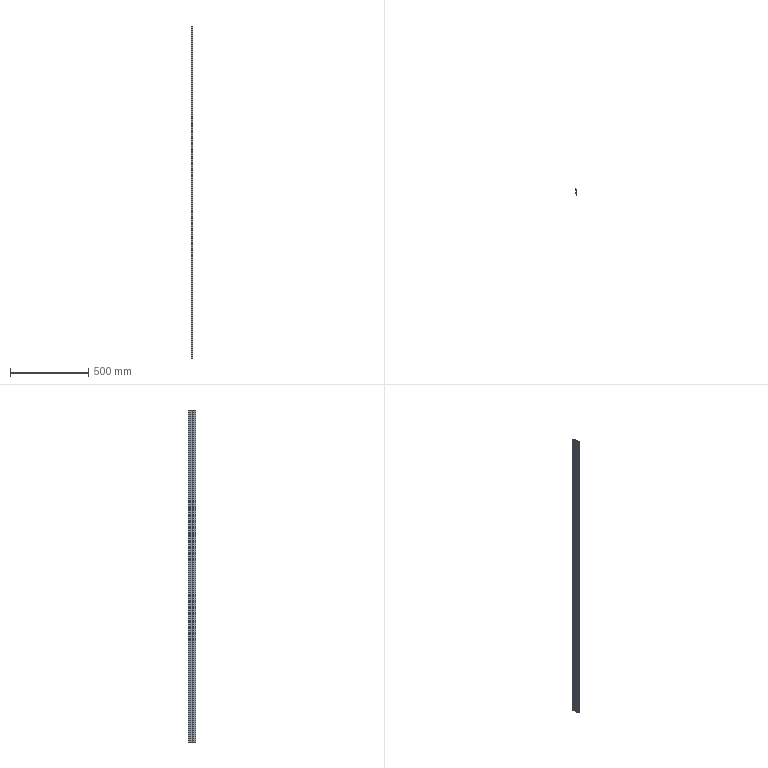Part | SolidWorks | features Extrusion 1 | 1 solid | 33 faces | box 9.4 x 46.998 x 2116 mm | volume 239025 mm3 | plane 22 | cylinder 11 | commonest cylinder face diameters 0.24 x2 0.4 x2 0.8 x2 1.2 x2 6 x2 1 x1
STEP:
#1=CARTESIAN_POINT('',(-2.9,32.45,-1058.));
#2=VERTEX_POINT('',#1);
#3=CARTESIAN_POINT('',(-2.7,32.25,-1058.));
#4=VERTEX_POINT('',#3);
#5=CARTESIAN_POINT('',(-2.7,32.45,-1058.));
#6=DIRECTION('',(0.,0.,1.));
#7=DIRECTION('',(1.,0.,0.));
#8=AXIS2_PLACEMENT_3D('',#5,#6,#7);
#9=CIRCLE('',#8,0.2);
#10=EDGE_CURVE('',#2,#4,#9,.T.);
#11=ORIENTED_EDGE('',*,*,#10,.T.);
#12=CARTESIAN_POINT('',(-2.7,32.25,1058.));
#13=VERTEX_POINT('',#12);
#14=CARTESIAN_POINT('',(-2.7,32.25,1058.));
#15=DIRECTION('',(0.,0.,-1.));
#16=VECTOR('',#15,1000.);
#17=LINE('',#14,#16);
#18=EDGE_CURVE('',#13,#4,#17,.T.);
#19=ORIENTED_EDGE('',*,*,#18,.F.);
#20=CARTESIAN_POINT('',(-2.9,32.45,1058.));
#21=VERTEX_POINT('',#20);
#22=CARTESIAN_POINT('',(-2.7,32.45,1058.));
#23=DIRECTION('',(0.,0.,1.));
#24=DIRECTION('',(1.,0.,0.));
#25=AXIS2_PLACEMENT_3D('',#22,#23,#24);
#26=CIRCLE('',#25,0.2);
#27=EDGE_CURVE('',#21,#13,#26,.T.);
#28=ORIENTED_EDGE('',*,*,#27,.F.);
#29=CARTESIAN_POINT('',(-2.9,32.45,1058.));
#30=DIRECTION('',(0.,0.,-1.));
#31=VECTOR('',#30,1000.);
#32=LINE('',#29,#31);
#33=EDGE_CURVE('',#21,#2,#32,.T.);
#34=ORIENTED_EDGE('',*,*,#33,.T.);
#35=EDGE_LOOP('',(#11,#19,#28,#34));
#36=FACE_OUTER_BOUND('',#35,.T.);
#37=CARTESIAN_POINT('',(-2.7,32.45,1058.));
#38=DIRECTION('',(0.,0.,-1.));
#39=DIRECTION('',(-1.,0.,0.));
#40=AXIS2_PLACEMENT_3D('',#37,#38,#39);
#41=CYLINDRICAL_SURFACE('',#40,0.2);
#42=ADVANCED_FACE('',(#36),#41,.T.);
#43=CARTESIAN_POINT('',(-2.5,32.25,-1058.));
#44=VERTEX_POINT('',#43);
#45=CARTESIAN_POINT('',(-2.7,32.25,-1058.));
#46=DIRECTION('',(1.,0.,0.));
#47=VECTOR('',#46,1000.);
#48=LINE('',#45,#47);
#49=EDGE_CURVE('',#4,#44,#48,.T.);
#50=ORIENTED_EDGE('',*,*,#49,.T.);
#51=CARTESIAN_POINT('',(-2.5,32.25,1058.));
#52=VERTEX_POINT('',#51);
#53=CARTESIAN_POINT('',(-2.5,32.25,1058.));
#54=DIRECTION('',(0.,0.,-1.));
#55=VECTOR('',#54,1000.);
#56=LINE('',#53,#55);
#57=EDGE_CURVE('',#52,#44,#56,.T.);
#58=ORIENTED_EDGE('',*,*,#57,.F.);
#59=CARTESIAN_POINT('',(-2.7,32.25,1058.));
#60=DIRECTION('',(1.,0.,0.));
#61=VECTOR('',#60,1000.);
#62=LINE('',#59,#61);
#63=EDGE_CURVE('',#13,#52,#62,.T.);
#64=ORIENTED_EDGE('',*,*,#63,.F.);
#65=ORIENTED_EDGE('',*,*,#18,.T.);
#66=EDGE_LOOP('',(#50,#58,#64,#65));
#67=FACE_OUTER_BOUND('',#66,.T.);
#68=CARTESIAN_POINT('',(-2.7,32.25,1058.));
#69=DIRECTION('',(0.,1.,0.));
#70=DIRECTION('',(0.,0.,1.));
#71=AXIS2_PLACEMENT_3D('',#68,#69,#70);
#72=PLANE('',#71);
#73=ADVANCED_FACE('',(#67),#72,.F.);
#74=CARTESIAN_POINT('',(-1.9,32.85,-1058.));
#75=VERTEX_POINT('',#74);
#76=CARTESIAN_POINT('',(-2.5,32.85,-1058.));
#77=DIRECTION('',(0.,0.,1.));
#78=DIRECTION('',(1.,0.,0.));
#79=AXIS2_PLACEMENT_3D('',#76,#77,#78);
#80=CIRCLE('',#79,0.6);
#81=EDGE_CURVE('',#44,#75,#80,.T.);
#82=ORIENTED_EDGE('',*,*,#81,.T.);
#83=CARTESIAN_POINT('',(-1.9,32.85,1058.));
#84=VERTEX_POINT('',#83);
#85=CARTESIAN_POINT('',(-1.9,32.85,1058.));
#86=DIRECTION('',(0.,0.,-1.));
#87=VECTOR('',#86,1000.);
#88=LINE('',#85,#87);
#89=EDGE_CURVE('',#84,#75,#88,.T.);
#90=ORIENTED_EDGE('',*,*,#89,.F.);
#91=CARTESIAN_POINT('',(-2.5,32.85,1058.));
#92=DIRECTION('',(0.,0.,1.));
#93=DIRECTION('',(1.,0.,0.));
#94=AXIS2_PLACEMENT_3D('',#91,#92,#93);
#95=CIRCLE('',#94,0.6);
#96=EDGE_CURVE('',#52,#84,#95,.T.);
#97=ORIENTED_EDGE('',*,*,#96,.F.);
#98=ORIENTED_EDGE('',*,*,#57,.T.);
#99=EDGE_LOOP('',(#82,#90,#97,#98));
#100=FACE_OUTER_BOUND('',#99,.T.);
#101=CARTESIAN_POINT('',(-2.5,32.85,1058.));
#102=DIRECTION('',(0.,0.,-1.));
#103=DIRECTION('',(-1.,0.,0.));
#104=AXIS2_PLACEMENT_3D('',#101,#102,#103);
#105=CYLINDRICAL_SURFACE('',#104,0.6);
#106=ADVANCED_FACE('',(#100),#105,.T.);
#107=CARTESIAN_POINT('',(-1.9,36.13,-1058.));
#108=VERTEX_POINT('',#107);
#109=CARTESIAN_POINT('',(-1.9,32.85,-1058.));
#110=DIRECTION('',(0.,1.,0.));
#111=VECTOR('',#110,1000.);
#112=LINE('',#109,#111);
#113=EDGE_CURVE('',#75,#108,#112,.T.);
#114=ORIENTED_EDGE('',*,*,#113,.T.);
#115=CARTESIAN_POINT('',(-1.9,36.13,1058.));
#116=VERTEX_POINT('',#115);
#117=CARTESIAN_POINT('',(-1.9,36.13,1058.));
#118=DIRECTION('',(0.,0.,-1.));
#119=VECTOR('',#118,1000.);
#120=LINE('',#117,#119);
#121=EDGE_CURVE('',#116,#108,#120,.T.);
#122=ORIENTED_EDGE('',*,*,#121,.F.);
#123=CARTESIAN_POINT('',(-1.9,32.85,1058.));
#124=DIRECTION('',(0.,1.,0.));
#125=VECTOR('',#124,1000.);
#126=LINE('',#123,#125);
#127=EDGE_CURVE('',#84,#116,#126,.T.);
#128=ORIENTED_EDGE('',*,*,#127,.F.);
#129=ORIENTED_EDGE('',*,*,#89,.T.);
#130=EDGE_LOOP('',(#114,#122,#128,#129));
#131=FACE_OUTER_BOUND('',#130,.T.);
#132=CARTESIAN_POINT('',(-1.9,32.85,1058.));
#133=DIRECTION('',(-1.,0.,0.));
#134=DIRECTION('',(0.,0.,1.));
#135=AXIS2_PLACEMENT_3D('',#132,#133,#134);
#136=PLANE('',#135);
#137=ADVANCED_FACE('',(#131),#136,.F.);
#138=CARTESIAN_POINT('',(-1.78,36.25,-1058.));
#139=VERTEX_POINT('',#138);
#140=CARTESIAN_POINT('',(-1.78,36.13,-1058.));
#141=DIRECTION('',(0.,0.,-1.));
#142=DIRECTION('',(1.,0.,0.));
#143=AXIS2_PLACEMENT_3D('',#140,#141,#142);
#144=CIRCLE('',#143,0.12);
#145=EDGE_CURVE('',#108,#139,#144,.T.);
#146=ORIENTED_EDGE('',*,*,#145,.T.);
#147=CARTESIAN_POINT('',(-1.78,36.25,1058.));
#148=VERTEX_POINT('',#147);
#149=CARTESIAN_POINT('',(-1.78,36.25,1058.));
#150=DIRECTION('',(0.,0.,-1.));
#151=VECTOR('',#150,1000.);
#152=LINE('',#149,#151);
#153=EDGE_CURVE('',#148,#139,#152,.T.);
#154=ORIENTED_EDGE('',*,*,#153,.F.);
#155=CARTESIAN_POINT('',(-1.78,36.13,1058.));
#156=DIRECTION('',(0.,0.,-1.));
#157=DIRECTION('',(1.,0.,0.));
#158=AXIS2_PLACEMENT_3D('',#155,#156,#157);
#159=CIRCLE('',#158,0.12);
#160=EDGE_CURVE('',#116,#148,#159,.T.);
#161=ORIENTED_EDGE('',*,*,#160,.F.);
#162=ORIENTED_EDGE('',*,*,#121,.T.);
#163=EDGE_LOOP('',(#146,#154,#161,#162));
#164=FACE_OUTER_BOUND('',#163,.T.);
#165=CARTESIAN_POINT('',(-1.78,36.13,1058.));
#166=DIRECTION('',(0.,0.,-1.));
#167=DIRECTION('',(-1.,0.,0.));
#168=AXIS2_PLACEMENT_3D('',#165,#166,#167);
#169=CYLINDRICAL_SURFACE('',#168,0.12);
#170=ADVANCED_FACE('',(#164),#169,.F.);
#171=CARTESIAN_POINT('',(0.,36.25,-1058.));
#172=VERTEX_POINT('',#171);
#173=CARTESIAN_POINT('',(-1.78,36.25,-1058.));
#174=DIRECTION('',(1.,0.,0.));
#175=VECTOR('',#174,1000.);
#176=LINE('',#173,#175);
#177=EDGE_CURVE('',#139,#172,#176,.T.);
#178=ORIENTED_EDGE('',*,*,#177,.T.);
#179=CARTESIAN_POINT('',(0.,36.25,1058.));
#180=VERTEX_POINT('',#179);
#181=CARTESIAN_POINT('',(0.,36.25,1058.));
#182=DIRECTION('',(0.,0.,-1.));
#183=VECTOR('',#182,1000.);
#184=LINE('',#181,#183);
#185=EDGE_CURVE('',#180,#172,#184,.T.);
#186=ORIENTED_EDGE('',*,*,#185,.F.);
#187=CARTESIAN_POINT('',(-1.78,36.25,1058.));
#188=DIRECTION('',(1.,0.,0.));
#189=VECTOR('',#188,1000.);
#190=LINE('',#187,#189);
#191=EDGE_CURVE('',#148,#180,#190,.T.);
#192=ORIENTED_EDGE('',*,*,#191,.F.);
#193=ORIENTED_EDGE('',*,*,#153,.T.);
#194=EDGE_LOOP('',(#178,#186,#192,#193));
#195=FACE_OUTER_BOUND('',#194,.T.);
#196=CARTESIAN_POINT('',(-1.78,36.25,1058.));
#197=DIRECTION('',(0.,1.,0.));
#198=DIRECTION('',(0.,0.,1.));
#199=AXIS2_PLACEMENT_3D('',#196,#197,#198);
#200=PLANE('',#199);
#201=ADVANCED_FACE('',(#195),#200,.F.);
#202=CARTESIAN_POINT('',(0.0007641,20.449,-1058.));
#203=VERTEX_POINT('',#202);
#204=CARTESIAN_POINT('',(0.,36.25,-1058.));
#205=DIRECTION('',(0.00004836,-1.,0.));
#206=VECTOR('',#205,1000.);
#207=LINE('',#204,#206);
#208=EDGE_CURVE('',#172,#203,#207,.T.);
#209=ORIENTED_EDGE('',*,*,#208,.T.);
#210=CARTESIAN_POINT('',(0.0007641,20.449,1058.));
#211=VERTEX_POINT('',#210);
#212=CARTESIAN_POINT('',(0.0007641,20.449,1058.));
#213=DIRECTION('',(0.,0.,-1.));
#214=VECTOR('',#213,1000.);
#215=LINE('',#212,#214);
#216=EDGE_CURVE('',#211,#203,#215,.T.);
#217=ORIENTED_EDGE('',*,*,#216,.F.);
#218=CARTESIAN_POINT('',(0.,36.25,1058.));
#219=DIRECTION('',(0.00004836,-1.,0.));
#220=VECTOR('',#219,1000.);
#221=LINE('',#218,#220);
#222=EDGE_CURVE('',#180,#211,#221,.T.);
#223=ORIENTED_EDGE('',*,*,#222,.F.);
#224=ORIENTED_EDGE('',*,*,#185,.T.);
#225=EDGE_LOOP('',(#209,#217,#223,#224));
#226=FACE_OUTER_BOUND('',#225,.T.);
#227=CARTESIAN_POINT('',(0.,36.25,1058.));
#228=DIRECTION('',(1.,0.00004836,0.));
#229=DIRECTION('',(-0.00004836,1.,0.));
#230=AXIS2_PLACEMENT_3D('',#227,#228,#229);
#231=PLANE('',#230);
#232=ADVANCED_FACE('',(#226),#231,.F.);
#233=CARTESIAN_POINT('',(-2.499,20.449,-1058.));
#234=VERTEX_POINT('',#233);
#235=CARTESIAN_POINT('',(0.0007641,20.449,-1058.));
#236=DIRECTION('',(-1.,0.,0.));
#237=VECTOR('',#236,1000.);
#238=LINE('',#235,#237);
#239=EDGE_CURVE('',#203,#234,#238,.T.);
#240=ORIENTED_EDGE('',*,*,#239,.T.);
#241=CARTESIAN_POINT('',(-2.499,20.449,1058.));
#242=VERTEX_POINT('',#241);
#243=CARTESIAN_POINT('',(-2.499,20.449,1058.));
#244=DIRECTION('',(0.,0.,-1.));
#245=VECTOR('',#244,1000.);
#246=LINE('',#243,#245);
#247=EDGE_CURVE('',#242,#234,#246,.T.);
#248=ORIENTED_EDGE('',*,*,#247,.F.);
#249=CARTESIAN_POINT('',(0.0007641,20.449,1058.));
#250=DIRECTION('',(-1.,0.,0.));
#251=VECTOR('',#250,1000.);
#252=LINE('',#249,#251);
#253=EDGE_CURVE('',#211,#242,#252,.T.);
#254=ORIENTED_EDGE('',*,*,#253,.F.);
#255=ORIENTED_EDGE('',*,*,#216,.T.);
#256=EDGE_LOOP('',(#240,#248,#254,#255));
#257=FACE_OUTER_BOUND('',#256,.T.);
#258=CARTESIAN_POINT('',(0.0007641,20.449,1058.));
#259=DIRECTION('',(0.,-1.,0.));
#260=DIRECTION('',(0.,0.,-1.));
#261=AXIS2_PLACEMENT_3D('',#258,#259,#260);
#262=PLANE('',#261);
#263=ADVANCED_FACE('',(#257),#262,.F.);
#264=CARTESIAN_POINT('',(-2.899,20.049,-1058.));
#265=VERTEX_POINT('',#264);
#266=CARTESIAN_POINT('',(-2.499,20.049,-1058.));
#267=DIRECTION('',(0.,0.,1.));
#268=DIRECTION('',(1.,0.,0.));
#269=AXIS2_PLACEMENT_3D('',#266,#267,#268);
#270=CIRCLE('',#269,0.4);
#271=EDGE_CURVE('',#234,#265,#270,.T.);
#272=ORIENTED_EDGE('',*,*,#271,.T.);
#273=CARTESIAN_POINT('',(-2.899,20.049,1058.));
#274=VERTEX_POINT('',#273);
#275=CARTESIAN_POINT('',(-2.899,20.049,1058.));
#276=DIRECTION('',(0.,0.,-1.));
#277=VECTOR('',#276,1000.);
#278=LINE('',#275,#277);
#279=EDGE_CURVE('',#274,#265,#278,.T.);
#280=ORIENTED_EDGE('',*,*,#279,.F.);
#281=CARTESIAN_POINT('',(-2.499,20.049,1058.));
#282=DIRECTION('',(0.,0.,1.));
#283=DIRECTION('',(1.,0.,0.));
#284=AXIS2_PLACEMENT_3D('',#281,#282,#283);
#285=CIRCLE('',#284,0.4);
#286=EDGE_CURVE('',#242,#274,#285,.T.);
#287=ORIENTED_EDGE('',*,*,#286,.F.);
#288=ORIENTED_EDGE('',*,*,#247,.T.);
#289=EDGE_LOOP('',(#272,#280,#287,#288));
#290=FACE_OUTER_BOUND('',#289,.T.);
#291=CARTESIAN_POINT('',(-2.499,20.049,1058.));
#292=DIRECTION('',(0.,0.,-1.));
#293=DIRECTION('',(-1.,0.,0.));
#294=AXIS2_PLACEMENT_3D('',#291,#292,#293);
#295=CYLINDRICAL_SURFACE('',#294,0.4);
#296=ADVANCED_FACE('',(#290),#295,.T.);
#297=CARTESIAN_POINT('',(-2.899,15.65,-1058.));
#298=VERTEX_POINT('',#297);
#299=CARTESIAN_POINT('',(-2.899,20.049,-1058.));
#300=DIRECTION('',(0.,-1.,0.));
#301=VECTOR('',#300,1000.);
#302=LINE('',#299,#301);
#303=EDGE_CURVE('',#265,#298,#302,.T.);
#304=ORIENTED_EDGE('',*,*,#303,.T.);
#305=CARTESIAN_POINT('',(-2.899,15.65,1058.));
#306=VERTEX_POINT('',#305);
#307=CARTESIAN_POINT('',(-2.899,15.65,1058.));
#308=DIRECTION('',(0.,0.,-1.));
#309=VECTOR('',#308,1000.);
#310=LINE('',#307,#309);
#311=EDGE_CURVE('',#306,#298,#310,.T.);
#312=ORIENTED_EDGE('',*,*,#311,.F.);
#313=CARTESIAN_POINT('',(-2.899,20.049,1058.));
#314=DIRECTION('',(0.,-1.,0.));
#315=VECTOR('',#314,1000.);
#316=LINE('',#313,#315);
#317=EDGE_CURVE('',#274,#306,#316,.T.);
#318=ORIENTED_EDGE('',*,*,#317,.F.);
#319=ORIENTED_EDGE('',*,*,#279,.T.);
#320=EDGE_LOOP('',(#304,#312,#318,#319));
#321=FACE_OUTER_BOUND('',#320,.T.);
#322=CARTESIAN_POINT('',(-2.899,20.049,1058.));
#323=DIRECTION('',(1.,0.,0.));
#324=DIRECTION('',(0.,0.,-1.));
#325=AXIS2_PLACEMENT_3D('',#322,#323,#324);
#326=PLANE('',#325);
#327=ADVANCED_FACE('',(#321),#326,.F.);
#328=CARTESIAN_POINT('',(-2.699,15.45,-1058.));
#329=VERTEX_POINT('',#328);
#330=CARTESIAN_POINT('',(-2.699,15.65,-1058.));
#331=DIRECTION('',(0.,0.,1.));
#332=DIRECTION('',(1.,0.,0.));
#333=AXIS2_PLACEMENT_3D('',#330,#331,#332);
#334=CIRCLE('',#333,0.2);
#335=EDGE_CURVE('',#298,#329,#334,.T.);
#336=ORIENTED_EDGE('',*,*,#335,.T.);
#337=CARTESIAN_POINT('',(-2.699,15.45,1058.));
#338=VERTEX_POINT('',#337);
#339=CARTESIAN_POINT('',(-2.699,15.45,1058.));
#340=DIRECTION('',(0.,0.,-1.));
#341=VECTOR('',#340,1000.);
#342=LINE('',#339,#341);
#343=EDGE_CURVE('',#338,#329,#342,.T.);
#344=ORIENTED_EDGE('',*,*,#343,.F.);
#345=CARTESIAN_POINT('',(-2.699,15.65,1058.));
#346=DIRECTION('',(0.,0.,1.));
#347=DIRECTION('',(1.,0.,0.));
#348=AXIS2_PLACEMENT_3D('',#345,#346,#347);
#349=CIRCLE('',#348,0.2);
#350=EDGE_CURVE('',#306,#338,#349,.T.);
#351=ORIENTED_EDGE('',*,*,#350,.F.);
#352=ORIENTED_EDGE('',*,*,#311,.T.);
#353=EDGE_LOOP('',(#336,#344,#351,#352));
#354=FACE_OUTER_BOUND('',#353,.T.);
#355=CARTESIAN_POINT('',(-2.699,15.65,1058.));
#356=DIRECTION('',(0.,0.,-1.));
#357=DIRECTION('',(-1.,0.,0.));
#358=AXIS2_PLACEMENT_3D('',#355,#356,#357);
#359=CYLINDRICAL_SURFACE('',#358,0.2);
#360=ADVANCED_FACE('',(#354),#359,.T.);
#361=CARTESIAN_POINT('',(-2.499,15.45,-1058.));
#362=VERTEX_POINT('',#361);
#363=CARTESIAN_POINT('',(-2.699,15.45,-1058.));
#364=DIRECTION('',(1.,0.,0.));
#365=VECTOR('',#364,1000.);
#366=LINE('',#363,#365);
#367=EDGE_CURVE('',#329,#362,#366,.T.);
#368=ORIENTED_EDGE('',*,*,#367,.T.);
#369=CARTESIAN_POINT('',(-2.499,15.45,1058.));
#370=VERTEX_POINT('',#369);
#371=CARTESIAN_POINT('',(-2.499,15.45,1058.));
#372=DIRECTION('',(0.,0.,-1.));
#373=VECTOR('',#372,1000.);
#374=LINE('',#371,#373);
#375=EDGE_CURVE('',#370,#362,#374,.T.);
#376=ORIENTED_EDGE('',*,*,#375,.F.);
#377=CARTESIAN_POINT('',(-2.699,15.45,1058.));
#378=DIRECTION('',(1.,0.,0.));
#379=VECTOR('',#378,1000.);
#380=LINE('',#377,#379);
#381=EDGE_CURVE('',#338,#370,#380,.T.);
#382=ORIENTED_EDGE('',*,*,#381,.F.);
#383=ORIENTED_EDGE('',*,*,#343,.T.);
#384=EDGE_LOOP('',(#368,#376,#382,#383));
#385=FACE_OUTER_BOUND('',#384,.T.);
#386=CARTESIAN_POINT('',(-2.699,15.45,1058.));
#387=DIRECTION('',(0.,1.,0.));
#388=DIRECTION('',(0.,0.,1.));
#389=AXIS2_PLACEMENT_3D('',#386,#387,#388);
#390=PLANE('',#389);
#391=ADVANCED_FACE('',(#385),#390,.F.);
#392=CARTESIAN_POINT('',(-1.899,16.05,-1058.));
#393=VERTEX_POINT('',#392);
#394=CARTESIAN_POINT('',(-2.499,16.05,-1058.));
#395=DIRECTION('',(0.,0.,1.));
#396=DIRECTION('',(1.,0.,0.));
#397=AXIS2_PLACEMENT_3D('',#394,#395,#396);
#398=CIRCLE('',#397,0.6);
#399=EDGE_CURVE('',#362,#393,#398,.T.);
#400=ORIENTED_EDGE('',*,*,#399,.T.);
#401=CARTESIAN_POINT('',(-1.899,16.05,1058.));
#402=VERTEX_POINT('',#401);
#403=CARTESIAN_POINT('',(-1.899,16.05,1058.));
#404=DIRECTION('',(0.,0.,-1.));
#405=VECTOR('',#404,1000.);
#406=LINE('',#403,#405);
#407=EDGE_CURVE('',#402,#393,#406,.T.);
#408=ORIENTED_EDGE('',*,*,#407,.F.);
#409=CARTESIAN_POINT('',(-2.499,16.05,1058.));
#410=DIRECTION('',(0.,0.,1.));
#411=DIRECTION('',(1.,0.,0.));
#412=AXIS2_PLACEMENT_3D('',#409,#410,#411);
#413=CIRCLE('',#412,0.6);
#414=EDGE_CURVE('',#370,#402,#413,.T.);
#415=ORIENTED_EDGE('',*,*,#414,.F.);
#416=ORIENTED_EDGE('',*,*,#375,.T.);
#417=EDGE_LOOP('',(#400,#408,#415,#416));
#418=FACE_OUTER_BOUND('',#417,.T.);
#419=CARTESIAN_POINT('',(-2.499,16.05,1058.));
#420=DIRECTION('',(0.,0.,-1.));
#421=DIRECTION('',(-1.,0.,0.));
#422=AXIS2_PLACEMENT_3D('',#419,#420,#421);
#423=CYLINDRICAL_SURFACE('',#422,0.6);
#424=ADVANCED_FACE('',(#418),#423,.T.);
#425=CARTESIAN_POINT('',(-1.899,19.329,-1058.));
#426=VERTEX_POINT('',#425);
#427=CARTESIAN_POINT('',(-1.899,16.05,-1058.));
#428=DIRECTION('',(0.,1.,0.));
#429=VECTOR('',#428,1000.);
#430=LINE('',#427,#429);
#431=EDGE_CURVE('',#393,#426,#430,.T.);
#432=ORIENTED_EDGE('',*,*,#431,.T.);
#433=CARTESIAN_POINT('',(-1.899,19.329,1058.));
#434=VERTEX_POINT('',#433);
#435=CARTESIAN_POINT('',(-1.899,19.329,1058.));
#436=DIRECTION('',(0.,0.,-1.));
#437=VECTOR('',#436,1000.);
#438=LINE('',#435,#437);
#439=EDGE_CURVE('',#434,#426,#438,.T.);
#440=ORIENTED_EDGE('',*,*,#439,.F.);
#441=CARTESIAN_POINT('',(-1.899,16.05,1058.));
#442=DIRECTION('',(0.,1.,0.));
#443=VECTOR('',#442,1000.);
#444=LINE('',#441,#443);
#445=EDGE_CURVE('',#402,#434,#444,.T.);
#446=ORIENTED_EDGE('',*,*,#445,.F.);
#447=ORIENTED_EDGE('',*,*,#407,.T.);
#448=EDGE_LOOP('',(#432,#440,#446,#447));
#449=FACE_OUTER_BOUND('',#448,.T.);
#450=CARTESIAN_POINT('',(-1.899,16.05,1058.));
#451=DIRECTION('',(-1.,0.,0.));
#452=DIRECTION('',(0.,0.,1.));
#453=AXIS2_PLACEMENT_3D('',#450,#451,#452);
#454=PLANE('',#453);
#455=ADVANCED_FACE('',(#449),#454,.F.);
#456=CARTESIAN_POINT('',(-1.779,19.449,-1058.));
#457=VERTEX_POINT('',#456);
#458=CARTESIAN_POINT('',(-1.779,19.329,-1058.));
#459=DIRECTION('',(0.,0.,-1.));
#460=DIRECTION('',(1.,0.,0.));
#461=AXIS2_PLACEMENT_3D('',#458,#459,#460);
#462=CIRCLE('',#461,0.12);
#463=EDGE_CURVE('',#426,#457,#462,.T.);
#464=ORIENTED_EDGE('',*,*,#463,.T.);
#465=CARTESIAN_POINT('',(-1.779,19.449,1058.));
#466=VERTEX_POINT('',#465);
#467=CARTESIAN_POINT('',(-1.779,19.449,1058.));
#468=DIRECTION('',(0.,0.,-1.));
#469=VECTOR('',#468,1000.);
#470=LINE('',#467,#469);
#471=EDGE_CURVE('',#466,#457,#470,.T.);
#472=ORIENTED_EDGE('',*,*,#471,.F.);
#473=CARTESIAN_POINT('',(-1.779,19.329,1058.));
#474=DIRECTION('',(0.,0.,-1.));
#475=DIRECTION('',(1.,0.,0.));
#476=AXIS2_PLACEMENT_3D('',#473,#474,#475);
#477=CIRCLE('',#476,0.12);
#478=EDGE_CURVE('',#434,#466,#477,.T.);
#479=ORIENTED_EDGE('',*,*,#478,.F.);
#480=ORIENTED_EDGE('',*,*,#439,.T.);
#481=EDGE_LOOP('',(#464,#472,#479,#480));
#482=FACE_OUTER_BOUND('',#481,.T.);
#483=CARTESIAN_POINT('',(-1.779,19.329,1058.));
#484=DIRECTION('',(0.,0.,-1.));
#485=DIRECTION('',(-1.,0.,0.));
#486=AXIS2_PLACEMENT_3D('',#483,#484,#485);
#487=CYLINDRICAL_SURFACE('',#486,0.12);
#488=ADVANCED_FACE('',(#482),#487,.F.);
#489=CARTESIAN_POINT('',(0.0007641,19.449,-1058.));
#490=VERTEX_POINT('',#489);
#491=CARTESIAN_POINT('',(-1.779,19.449,-1058.));
#492=DIRECTION('',(1.,0.,0.));
#493=VECTOR('',#492,1000.);
#494=LINE('',#491,#493);
#495=EDGE_CURVE('',#457,#490,#494,.T.);
#496=ORIENTED_EDGE('',*,*,#495,.T.);
#497=CARTESIAN_POINT('',(0.0007641,19.449,1058.));
#498=VERTEX_POINT('',#497);
#499=CARTESIAN_POINT('',(0.0007641,19.449,1058.));
#500=DIRECTION('',(0.,0.,-1.));
#501=VECTOR('',#500,1000.);
#502=LINE('',#499,#501);
#503=EDGE_CURVE('',#498,#490,#502,.T.);
#504=ORIENTED_EDGE('',*,*,#503,.F.);
#505=CARTESIAN_POINT('',(-1.779,19.449,1058.));
#506=DIRECTION('',(1.,0.,0.));
#507=VECTOR('',#506,1000.);
#508=LINE('',#505,#507);
#509=EDGE_CURVE('',#466,#498,#508,.T.);
#510=ORIENTED_EDGE('',*,*,#509,.F.);
#511=ORIENTED_EDGE('',*,*,#471,.T.);
#512=EDGE_LOOP('',(#496,#504,#510,#511));
#513=FACE_OUTER_BOUND('',#512,.T.);
#514=CARTESIAN_POINT('',(-1.779,19.449,1058.));
#515=DIRECTION('',(0.,1.,0.));
#516=DIRECTION('',(0.,0.,1.));
#517=AXIS2_PLACEMENT_3D('',#514,#515,#516);
#518=PLANE('',#517);
#519=ADVANCED_FACE('',(#513),#518,.F.);
#520=CARTESIAN_POINT('',(0.,0.,-1058.));
#521=VERTEX_POINT('',#520);
#522=CARTESIAN_POINT('',(0.0007641,19.449,-1058.));
#523=DIRECTION('',(-0.00003929,-1.,0.));
#524=VECTOR('',#523,1000.);
#525=LINE('',#522,#524);
#526=EDGE_CURVE('',#490,#521,#525,.T.);
#527=ORIENTED_EDGE('',*,*,#526,.T.);
#528=CARTESIAN_POINT('',(0.,0.,1058.));
#529=VERTEX_POINT('',#528);
#530=CARTESIAN_POINT('',(0.,0.,1058.));
#531=DIRECTION('',(0.,0.,-1.));
#532=VECTOR('',#531,1000.);
#533=LINE('',#530,#532);
#534=EDGE_CURVE('',#529,#521,#533,.T.);
#535=ORIENTED_EDGE('',*,*,#534,.F.);
#536=CARTESIAN_POINT('',(0.0007641,19.449,1058.));
#537=DIRECTION('',(-0.00003929,-1.,0.));
#538=VECTOR('',#537,1000.);
#539=LINE('',#536,#538);
#540=EDGE_CURVE('',#498,#529,#539,.T.);
#541=ORIENTED_EDGE('',*,*,#540,.F.);
#542=ORIENTED_EDGE('',*,*,#503,.T.);
#543=EDGE_LOOP('',(#527,#535,#541,#542));
#544=FACE_OUTER_BOUND('',#543,.T.);
#545=CARTESIAN_POINT('',(0.0007641,19.449,1058.));
#546=DIRECTION('',(1.,-0.00003929,0.));
#547=DIRECTION('',(0.00003929,1.,0.));
#548=AXIS2_PLACEMENT_3D('',#545,#546,#547);
#549=PLANE('',#548);
#550=ADVANCED_FACE('',(#544),#549,.F.);
#551=CARTESIAN_POINT('',(1.5,0.,-1058.));
#552=VERTEX_POINT('',#551);
#553=CARTESIAN_POINT('',(0.,0.,-1058.));
#554=DIRECTION('',(1.,0.,0.));
#555=VECTOR('',#554,1000.);
#556=LINE('',#553,#555);
#557=EDGE_CURVE('',#521,#552,#556,.T.);
#558=ORIENTED_EDGE('',*,*,#557,.T.);
#559=CARTESIAN_POINT('',(1.5,0.,1058.));
#560=VERTEX_POINT('',#559);
#561=CARTESIAN_POINT('',(1.5,0.,1058.));
#562=DIRECTION('',(0.,0.,-1.));
#563=VECTOR('',#562,1000.);
#564=LINE('',#561,#563);
#565=EDGE_CURVE('',#560,#552,#564,.T.);
#566=ORIENTED_EDGE('',*,*,#565,.F.);
#567=CARTESIAN_POINT('',(0.,0.,1058.));
#568=DIRECTION('',(1.,0.,0.));
#569=VECTOR('',#568,1000.);
#570=LINE('',#567,#569);
#571=EDGE_CURVE('',#529,#560,#570,.T.);
#572=ORIENTED_EDGE('',*,*,#571,.F.);
#573=ORIENTED_EDGE('',*,*,#534,.T.);
#574=EDGE_LOOP('',(#558,#566,#572,#573));
#575=FACE_OUTER_BOUND('',#574,.T.);
#576=CARTESIAN_POINT('',(0.,0.,1058.));
#577=DIRECTION('',(0.,1.,0.));
#578=DIRECTION('',(0.,0.,1.));
#579=AXIS2_PLACEMENT_3D('',#576,#577,#578);
#580=PLANE('',#579);
#581=ADVANCED_FACE('',(#575),#580,.F.);
#582=CARTESIAN_POINT('',(2.,0.5,-1058.));
#583=VERTEX_POINT('',#582);
#584=CARTESIAN_POINT('',(1.5,0.5,-1058.));
#585=DIRECTION('',(0.,0.,1.));
#586=DIRECTION('',(1.,0.,0.));
#587=AXIS2_PLACEMENT_3D('',#584,#585,#586);
#588=CIRCLE('',#587,0.5);
#589=EDGE_CURVE('',#552,#583,#588,.T.);
#590=ORIENTED_EDGE('',*,*,#589,.T.);
#591=CARTESIAN_POINT('',(2.,0.5,1058.));
#592=VERTEX_POINT('',#591);
#593=CARTESIAN_POINT('',(2.,0.5,1058.));
#594=DIRECTION('',(0.,0.,-1.));
#595=VECTOR('',#594,1000.);
#596=LINE('',#593,#595);
#597=EDGE_CURVE('',#592,#583,#596,.T.);
#598=ORIENTED_EDGE('',*,*,#597,.F.);
#599=CARTESIAN_POINT('',(1.5,0.5,1058.));
#600=DIRECTION('',(0.,0.,1.));
#601=DIRECTION('',(1.,0.,0.));
#602=AXIS2_PLACEMENT_3D('',#599,#600,#601);
#603=CIRCLE('',#602,0.5);
#604=EDGE_CURVE('',#560,#592,#603,.T.);
#605=ORIENTED_EDGE('',*,*,#604,.F.);
#606=ORIENTED_EDGE('',*,*,#565,.T.);
#607=EDGE_LOOP('',(#590,#598,#605,#606));
#608=FACE_OUTER_BOUND('',#607,.T.);
#609=CARTESIAN_POINT('',(1.5,0.5,1058.));
#610=DIRECTION('',(0.,0.,-1.));
#611=DIRECTION('',(-1.,0.,0.));
#612=AXIS2_PLACEMENT_3D('',#609,#610,#611);
#613=CYLINDRICAL_SURFACE('',#612,0.5);
#614=ADVANCED_FACE('',(#608),#613,.T.);
#615=CARTESIAN_POINT('',(2.,38.058,-1058.));
#616=VERTEX_POINT('',#615);
#617=CARTESIAN_POINT('',(2.,0.5,-1058.));
#618=DIRECTION('',(0.,1.,0.));
#619=VECTOR('',#618,1000.);
#620=LINE('',#617,#619);
#621=EDGE_CURVE('',#583,#616,#620,.T.);
#622=ORIENTED_EDGE('',*,*,#621,.T.);
#623=CARTESIAN_POINT('',(2.,38.058,1058.));
#624=VERTEX_POINT('',#623);
#625=CARTESIAN_POINT('',(2.,38.058,1058.));
#626=DIRECTION('',(0.,0.,-1.));
#627=VECTOR('',#626,1000.);
#628=LINE('',#625,#627);
#629=EDGE_CURVE('',#624,#616,#628,.T.);
#630=ORIENTED_EDGE('',*,*,#629,.F.);
#631=CARTESIAN_POINT('',(2.,0.5,1058.));
#632=DIRECTION('',(0.,1.,0.));
#633=VECTOR('',#632,1000.);
#634=LINE('',#631,#633);
#635=EDGE_CURVE('',#592,#624,#634,.T.);
#636=ORIENTED_EDGE('',*,*,#635,.F.);
#637=ORIENTED_EDGE('',*,*,#597,.T.);
#638=EDGE_LOOP('',(#622,#630,#636,#637));
#639=FACE_OUTER_BOUND('',#638,.T.);
#640=CARTESIAN_POINT('',(2.,0.5,1058.));
#641=DIRECTION('',(-1.,0.,0.));
#642=DIRECTION('',(0.,0.,1.));
#643=AXIS2_PLACEMENT_3D('',#640,#641,#642);
#644=PLANE('',#643);
#645=ADVANCED_FACE('',(#639),#644,.F.);
#646=CARTESIAN_POINT('',(1.393,39.868,-1058.));
#647=VERTEX_POINT('',#646);
#648=CARTESIAN_POINT('',(-1.,38.058,-1058.));
#649=DIRECTION('',(0.,0.,1.));
#650=DIRECTION('',(1.,0.,0.));
#651=AXIS2_PLACEMENT_3D('',#648,#649,#650);
#652=CIRCLE('',#651,3.);
#653=EDGE_CURVE('',#616,#647,#652,.T.);
#654=ORIENTED_EDGE('',*,*,#653,.T.);
#655=CARTESIAN_POINT('',(1.393,39.868,1058.));
#656=VERTEX_POINT('',#655);
#657=CARTESIAN_POINT('',(1.393,39.868,1058.));
#658=DIRECTION('',(0.,0.,-1.));
#659=VECTOR('',#658,1000.);
#660=LINE('',#657,#659);
#661=EDGE_CURVE('',#656,#647,#660,.T.);
#662=ORIENTED_EDGE('',*,*,#661,.F.);
#663=CARTESIAN_POINT('',(-1.,38.058,1058.));
#664=DIRECTION('',(0.,0.,1.));
#665=DIRECTION('',(1.,0.,0.));
#666=AXIS2_PLACEMENT_3D('',#663,#664,#665);
#667=CIRCLE('',#666,3.);
#668=EDGE_CURVE('',#624,#656,#667,.T.);
#669=ORIENTED_EDGE('',*,*,#668,.F.);
#670=ORIENTED_EDGE('',*,*,#629,.T.);
#671=EDGE_LOOP('',(#654,#662,#669,#670));
#672=FACE_OUTER_BOUND('',#671,.T.);
#673=CARTESIAN_POINT('',(-1.,38.058,1058.));
#674=DIRECTION('',(0.,0.,-1.));
#675=DIRECTION('',(-1.,0.,0.));
#676=AXIS2_PLACEMENT_3D('',#673,#674,#675);
#677=CYLINDRICAL_SURFACE('',#676,3.);
#678=ADVANCED_FACE('',(#672),#677,.T.);
#679=CARTESIAN_POINT('',(-4.,46.998,-1058.));
#680=VERTEX_POINT('',#679);
#681=CARTESIAN_POINT('',(1.393,39.868,-1058.));
#682=DIRECTION('',(-0.6032,0.7976,0.));
#683=VECTOR('',#682,1000.);
#684=LINE('',#681,#683);
#685=EDGE_CURVE('',#647,#680,#684,.T.);
#686=ORIENTED_EDGE('',*,*,#685,.T.);
#687=CARTESIAN_POINT('',(-4.,46.998,1058.));
#688=VERTEX_POINT('',#687);
#689=CARTESIAN_POINT('',(-4.,46.998,1058.));
#690=DIRECTION('',(0.,0.,-1.));
#691=VECTOR('',#690,1000.);
#692=LINE('',#689,#691);
#693=EDGE_CURVE('',#688,#680,#692,.T.);
#694=ORIENTED_EDGE('',*,*,#693,.F.);
#695=CARTESIAN_POINT('',(1.393,39.868,1058.));
#696=DIRECTION('',(-0.6032,0.7976,0.));
#697=VECTOR('',#696,1000.);
#698=LINE('',#695,#697);
#699=EDGE_CURVE('',#656,#688,#698,.T.);
#700=ORIENTED_EDGE('',*,*,#699,.F.);
#701=ORIENTED_EDGE('',*,*,#661,.T.);
#702=EDGE_LOOP('',(#686,#694,#700,#701));
#703=FACE_OUTER_BOUND('',#702,.T.);
#704=CARTESIAN_POINT('',(1.393,39.868,1058.));
#705=DIRECTION('',(-0.7976,-0.6032,0.));
#706=DIRECTION('',(0.6032,-0.7976,0.));
#707=AXIS2_PLACEMENT_3D('',#704,#705,#706);
#708=PLANE('',#707);
#709=ADVANCED_FACE('',(#703),#708,.F.);
#710=CARTESIAN_POINT('',(-7.4,46.998,-1058.));
#711=VERTEX_POINT('',#710);
#712=CARTESIAN_POINT('',(-4.,46.998,-1058.));
#713=DIRECTION('',(-1.,0.,0.));
#714=VECTOR('',#713,1000.);
#715=LINE('',#712,#714);
#716=EDGE_CURVE('',#680,#711,#715,.T.);
#717=ORIENTED_EDGE('',*,*,#716,.T.);
#718=CARTESIAN_POINT('',(-7.4,46.998,1058.));
#719=VERTEX_POINT('',#718);
#720=CARTESIAN_POINT('',(-7.4,46.998,1058.));
#721=DIRECTION('',(0.,0.,-1.));
#722=VECTOR('',#721,1000.);
#723=LINE('',#720,#722);
#724=EDGE_CURVE('',#719,#711,#723,.T.);
#725=ORIENTED_EDGE('',*,*,#724,.F.);
#726=CARTESIAN_POINT('',(-4.,46.998,1058.));
#727=DIRECTION('',(-1.,0.,0.));
#728=VECTOR('',#727,1000.);
#729=LINE('',#726,#728);
#730=EDGE_CURVE('',#688,#719,#729,.T.);
#731=ORIENTED_EDGE('',*,*,#730,.F.);
#732=ORIENTED_EDGE('',*,*,#693,.T.);
#733=EDGE_LOOP('',(#717,#725,#731,#732));
#734=FACE_OUTER_BOUND('',#733,.T.);
#735=CARTESIAN_POINT('',(-4.,46.998,1058.));
#736=DIRECTION('',(0.,-1.,0.));
#737=DIRECTION('',(0.,0.,-1.));
#738=AXIS2_PLACEMENT_3D('',#735,#736,#737);
#739=PLANE('',#738);
#740=ADVANCED_FACE('',(#734),#739,.F.);
#741=CARTESIAN_POINT('',(-7.4,45.998,-1058.));
#742=VERTEX_POINT('',#741);
#743=CARTESIAN_POINT('',(-7.4,46.998,-1058.));
#744=DIRECTION('',(0.,-1.,0.));
#745=VECTOR('',#744,1000.);
#746=LINE('',#743,#745);
#747=EDGE_CURVE('',#711,#742,#746,.T.);
#748=ORIENTED_EDGE('',*,*,#747,.T.);
#749=CARTESIAN_POINT('',(-7.4,45.998,1058.));
#750=VERTEX_POINT('',#749);
#751=CARTESIAN_POINT('',(-7.4,45.998,1058.));
#752=DIRECTION('',(0.,0.,-1.));
#753=VECTOR('',#752,1000.);
#754=LINE('',#751,#753);
#755=EDGE_CURVE('',#750,#742,#754,.T.);
#756=ORIENTED_EDGE('',*,*,#755,.F.);
#757=CARTESIAN_POINT('',(-7.4,46.998,1058.));
#758=DIRECTION('',(0.,-1.,0.));
#759=VECTOR('',#758,1000.);
#760=LINE('',#757,#759);
#761=EDGE_CURVE('',#719,#750,#760,.T.);
#762=ORIENTED_EDGE('',*,*,#761,.F.);
#763=ORIENTED_EDGE('',*,*,#724,.T.);
#764=EDGE_LOOP('',(#748,#756,#762,#763));
#765=FACE_OUTER_BOUND('',#764,.T.);
#766=CARTESIAN_POINT('',(-7.4,46.998,1058.));
#767=DIRECTION('',(1.,0.,0.));
#768=DIRECTION('',(0.,0.,-1.));
#769=AXIS2_PLACEMENT_3D('',#766,#767,#768);
#770=PLANE('',#769);
#771=ADVANCED_FACE('',(#765),#770,.F.);
#772=CARTESIAN_POINT('',(-5.751,45.998,-1058.));
#773=VERTEX_POINT('',#772);
#774=CARTESIAN_POINT('',(-7.4,45.998,-1058.));
#775=DIRECTION('',(1.,0.,0.));
#776=VECTOR('',#775,1000.);
#777=LINE('',#774,#776);
#778=EDGE_CURVE('',#742,#773,#777,.T.);
#779=ORIENTED_EDGE('',*,*,#778,.T.);
#780=CARTESIAN_POINT('',(-5.751,45.998,1058.));
#781=VERTEX_POINT('',#780);
#782=CARTESIAN_POINT('',(-5.751,45.998,1058.));
#783=DIRECTION('',(0.,0.,-1.));
#784=VECTOR('',#783,1000.);
#785=LINE('',#782,#784);
#786=EDGE_CURVE('',#781,#773,#785,.T.);
#787=ORIENTED_EDGE('',*,*,#786,.F.);
#788=CARTESIAN_POINT('',(-7.4,45.998,1058.));
#789=DIRECTION('',(1.,0.,0.));
#790=VECTOR('',#789,1000.);
#791=LINE('',#788,#790);
#792=EDGE_CURVE('',#750,#781,#791,.T.);
#793=ORIENTED_EDGE('',*,*,#792,.F.);
#794=ORIENTED_EDGE('',*,*,#755,.T.);
#795=EDGE_LOOP('',(#779,#787,#793,#794));
#796=FACE_OUTER_BOUND('',#795,.T.);
#797=CARTESIAN_POINT('',(-7.4,45.998,1058.));
#798=DIRECTION('',(0.,1.,0.));
#799=DIRECTION('',(0.,0.,1.));
#800=AXIS2_PLACEMENT_3D('',#797,#798,#799);
#801=PLANE('',#800);
#802=ADVANCED_FACE('',(#796),#801,.F.);
#803=CARTESIAN_POINT('',(-0.6072,39.196,-1058.));
#804=VERTEX_POINT('',#803);
#805=CARTESIAN_POINT('',(-5.751,45.998,-1058.));
#806=DIRECTION('',(0.6032,-0.7976,0.));
#807=VECTOR('',#806,1000.);
#808=LINE('',#805,#807);
#809=EDGE_CURVE('',#773,#804,#808,.T.);
#810=ORIENTED_EDGE('',*,*,#809,.T.);
#811=CARTESIAN_POINT('',(-0.6072,39.196,1058.));
#812=VERTEX_POINT('',#811);
#813=CARTESIAN_POINT('',(-0.6072,39.196,1058.));
#814=DIRECTION('',(0.,0.,-1.));
#815=VECTOR('',#814,1000.);
#816=LINE('',#813,#815);
#817=EDGE_CURVE('',#812,#804,#816,.T.);
#818=ORIENTED_EDGE('',*,*,#817,.F.);
#819=CARTESIAN_POINT('',(-5.751,45.998,1058.));
#820=DIRECTION('',(0.6032,-0.7976,0.));
#821=VECTOR('',#820,1000.);
#822=LINE('',#819,#821);
#823=EDGE_CURVE('',#781,#812,#822,.T.);
#824=ORIENTED_EDGE('',*,*,#823,.F.);
#825=ORIENTED_EDGE('',*,*,#786,.T.);
#826=EDGE_LOOP('',(#810,#818,#824,#825));
#827=FACE_OUTER_BOUND('',#826,.T.);
#828=CARTESIAN_POINT('',(-5.751,45.998,1058.));
#829=DIRECTION('',(0.7976,0.6032,0.));
#830=DIRECTION('',(-0.6032,0.7976,0.));
#831=AXIS2_PLACEMENT_3D('',#828,#829,#830);
#832=PLANE('',#831);
#833=ADVANCED_FACE('',(#827),#832,.F.);
#834=CARTESIAN_POINT('',(0.,37.387,-1058.));
#835=VERTEX_POINT('',#834);
#836=CARTESIAN_POINT('',(-3.,37.387,-1058.));
#837=DIRECTION('',(0.,0.,-1.));
#838=DIRECTION('',(1.,0.,0.));
#839=AXIS2_PLACEMENT_3D('',#836,#837,#838);
#840=CIRCLE('',#839,3.);
#841=EDGE_CURVE('',#804,#835,#840,.T.);
#842=ORIENTED_EDGE('',*,*,#841,.T.);
#843=CARTESIAN_POINT('',(0.,37.387,1058.));
#844=VERTEX_POINT('',#843);
#845=CARTESIAN_POINT('',(0.,37.387,1058.));
#846=DIRECTION('',(0.,0.,-1.));
#847=VECTOR('',#846,1000.);
#848=LINE('',#845,#847);
#849=EDGE_CURVE('',#844,#835,#848,.T.);
#850=ORIENTED_EDGE('',*,*,#849,.F.);
#851=CARTESIAN_POINT('',(-3.,37.387,1058.));
#852=DIRECTION('',(0.,0.,-1.));
#853=DIRECTION('',(1.,0.,0.));
#854=AXIS2_PLACEMENT_3D('',#851,#852,#853);
#855=CIRCLE('',#854,3.);
#856=EDGE_CURVE('',#812,#844,#855,.T.);
#857=ORIENTED_EDGE('',*,*,#856,.F.);
#858=ORIENTED_EDGE('',*,*,#817,.T.);
#859=EDGE_LOOP('',(#842,#850,#857,#858));
#860=FACE_OUTER_BOUND('',#859,.T.);
#861=CARTESIAN_POINT('',(-3.,37.387,1058.));
#862=DIRECTION('',(0.,0.,-1.));
#863=DIRECTION('',(-1.,0.,0.));
#864=AXIS2_PLACEMENT_3D('',#861,#862,#863);
#865=CYLINDRICAL_SURFACE('',#864,3.);
#866=ADVANCED_FACE('',(#860),#865,.F.);
#867=CARTESIAN_POINT('',(0.,37.25,-1058.));
#868=VERTEX_POINT('',#867);
#869=CARTESIAN_POINT('',(0.,37.387,-1058.));
#870=DIRECTION('',(0.,-1.,0.));
#871=VECTOR('',#870,1000.);
#872=LINE('',#869,#871);
#873=EDGE_CURVE('',#835,#868,#872,.T.);
#874=ORIENTED_EDGE('',*,*,#873,.T.);
#875=CARTESIAN_POINT('',(0.,37.25,1058.));
#876=VERTEX_POINT('',#875);
#877=CARTESIAN_POINT('',(0.,37.25,1058.));
#878=DIRECTION('',(0.,0.,-1.));
#879=VECTOR('',#878,1000.);
#880=LINE('',#877,#879);
#881=EDGE_CURVE('',#876,#868,#880,.T.);
#882=ORIENTED_EDGE('',*,*,#881,.F.);
#883=CARTESIAN_POINT('',(0.,37.387,1058.));
#884=DIRECTION('',(0.,-1.,0.));
#885=VECTOR('',#884,1000.);
#886=LINE('',#883,#885);
#887=EDGE_CURVE('',#844,#876,#886,.T.);
#888=ORIENTED_EDGE('',*,*,#887,.F.);
#889=ORIENTED_EDGE('',*,*,#849,.T.);
#890=EDGE_LOOP('',(#874,#882,#888,#889));
#891=FACE_OUTER_BOUND('',#890,.T.);
#892=CARTESIAN_POINT('',(0.,37.387,1058.));
#893=DIRECTION('',(1.,0.,0.));
#894=DIRECTION('',(0.,1.,0.));
#895=AXIS2_PLACEMENT_3D('',#892,#893,#894);
#896=PLANE('',#895);
#897=ADVANCED_FACE('',(#891),#896,.F.);
#898=CARTESIAN_POINT('',(-2.5,37.25,-1058.));
#899=VERTEX_POINT('',#898);
#900=CARTESIAN_POINT('',(0.,37.25,-1058.));
#901=DIRECTION('',(-1.,0.,0.));
#902=VECTOR('',#901,1000.);
#903=LINE('',#900,#902);
#904=EDGE_CURVE('',#868,#899,#903,.T.);
#905=ORIENTED_EDGE('',*,*,#904,.T.);
#906=CARTESIAN_POINT('',(-2.5,37.25,1058.));
#907=VERTEX_POINT('',#906);
#908=CARTESIAN_POINT('',(-2.5,37.25,1058.));
#909=DIRECTION('',(0.,0.,-1.));
#910=VECTOR('',#909,1000.);
#911=LINE('',#908,#910);
#912=EDGE_CURVE('',#907,#899,#911,.T.);
#913=ORIENTED_EDGE('',*,*,#912,.F.);
#914=CARTESIAN_POINT('',(0.,37.25,1058.));
#915=DIRECTION('',(-1.,0.,0.));
#916=VECTOR('',#915,1000.);
#917=LINE('',#914,#916);
#918=EDGE_CURVE('',#876,#907,#917,.T.);
#919=ORIENTED_EDGE('',*,*,#918,.F.);
#920=ORIENTED_EDGE('',*,*,#881,.T.);
#921=EDGE_LOOP('',(#905,#913,#919,#920));
#922=FACE_OUTER_BOUND('',#921,.T.);
#923=CARTESIAN_POINT('',(0.,37.25,1058.));
#924=DIRECTION('',(0.,-1.,0.));
#925=DIRECTION('',(0.,0.,-1.));
#926=AXIS2_PLACEMENT_3D('',#923,#924,#925);
#927=PLANE('',#926);
#928=ADVANCED_FACE('',(#922),#927,.F.);
#929=CARTESIAN_POINT('',(-2.9,36.85,-1058.));
#930=VERTEX_POINT('',#929);
#931=CARTESIAN_POINT('',(-2.5,36.85,-1058.));
#932=DIRECTION('',(0.,0.,1.));
#933=DIRECTION('',(1.,0.,0.));
#934=AXIS2_PLACEMENT_3D('',#931,#932,#933);
#935=CIRCLE('',#934,0.4);
#936=EDGE_CURVE('',#899,#930,#935,.T.);
#937=ORIENTED_EDGE('',*,*,#936,.T.);
#938=CARTESIAN_POINT('',(-2.9,36.85,1058.));
#939=VERTEX_POINT('',#938);
#940=CARTESIAN_POINT('',(-2.9,36.85,1058.));
#941=DIRECTION('',(0.,0.,-1.));
#942=VECTOR('',#941,1000.);
#943=LINE('',#940,#942);
#944=EDGE_CURVE('',#939,#930,#943,.T.);
#945=ORIENTED_EDGE('',*,*,#944,.F.);
#946=CARTESIAN_POINT('',(-2.5,36.85,1058.));
#947=DIRECTION('',(0.,0.,1.));
#948=DIRECTION('',(1.,0.,0.));
#949=AXIS2_PLACEMENT_3D('',#946,#947,#948);
#950=CIRCLE('',#949,0.4);
#951=EDGE_CURVE('',#907,#939,#950,.T.);
#952=ORIENTED_EDGE('',*,*,#951,.F.);
#953=ORIENTED_EDGE('',*,*,#912,.T.);
#954=EDGE_LOOP('',(#937,#945,#952,#953));
#955=FACE_OUTER_BOUND('',#954,.T.);
#956=CARTESIAN_POINT('',(-2.5,36.85,1058.));
#957=DIRECTION('',(0.,0.,-1.));
#958=DIRECTION('',(-1.,0.,0.));
#959=AXIS2_PLACEMENT_3D('',#956,#957,#958);
#960=CYLINDRICAL_SURFACE('',#959,0.4);
#961=ADVANCED_FACE('',(#955),#960,.T.);
#962=CARTESIAN_POINT('',(-2.9,36.85,-1058.));
#963=DIRECTION('',(0.,-1.,0.));
#964=VECTOR('',#963,1000.);
#965=LINE('',#962,#964);
#966=EDGE_CURVE('',#930,#2,#965,.T.);
#967=ORIENTED_EDGE('',*,*,#966,.T.);
#968=ORIENTED_EDGE('',*,*,#33,.F.);
#969=CARTESIAN_POINT('',(-2.9,36.85,1058.));
#970=DIRECTION('',(0.,-1.,0.));
#971=VECTOR('',#970,1000.);
#972=LINE('',#969,#971);
#973=EDGE_CURVE('',#939,#21,#972,.T.);
#974=ORIENTED_EDGE('',*,*,#973,.F.);
#975=ORIENTED_EDGE('',*,*,#944,.T.);
#976=EDGE_LOOP('',(#967,#968,#974,#975));
#977=FACE_OUTER_BOUND('',#976,.T.);
#978=CARTESIAN_POINT('',(-2.9,36.85,1058.));
#979=DIRECTION('',(1.,0.,0.));
#980=DIRECTION('',(0.,0.,-1.));
#981=AXIS2_PLACEMENT_3D('',#978,#979,#980);
#982=PLANE('',#981);
#983=ADVANCED_FACE('',(#977),#982,.F.);
#984=ORIENTED_EDGE('',*,*,#27,.T.);
#985=ORIENTED_EDGE('',*,*,#63,.T.);
#986=ORIENTED_EDGE('',*,*,#96,.T.);
#987=ORIENTED_EDGE('',*,*,#127,.T.);
#988=ORIENTED_EDGE('',*,*,#160,.T.);
#989=ORIENTED_EDGE('',*,*,#191,.T.);
#990=ORIENTED_EDGE('',*,*,#222,.T.);
#991=ORIENTED_EDGE('',*,*,#253,.T.);
#992=ORIENTED_EDGE('',*,*,#286,.T.);
#993=ORIENTED_EDGE('',*,*,#317,.T.);
#994=ORIENTED_EDGE('',*,*,#350,.T.);
#995=ORIENTED_EDGE('',*,*,#381,.T.);
#996=ORIENTED_EDGE('',*,*,#414,.T.);
#997=ORIENTED_EDGE('',*,*,#445,.T.);
#998=ORIENTED_EDGE('',*,*,#478,.T.);
#999=ORIENTED_EDGE('',*,*,#509,.T.);
#1000=ORIENTED_EDGE('',*,*,#540,.T.);
#1001=ORIENTED_EDGE('',*,*,#571,.T.);
#1002=ORIENTED_EDGE('',*,*,#604,.T.);
#1003=ORIENTED_EDGE('',*,*,#635,.T.);
#1004=ORIENTED_EDGE('',*,*,#668,.T.);
#1005=ORIENTED_EDGE('',*,*,#699,.T.);
#1006=ORIENTED_EDGE('',*,*,#730,.T.);
#1007=ORIENTED_EDGE('',*,*,#761,.T.);
#1008=ORIENTED_EDGE('',*,*,#792,.T.);
#1009=ORIENTED_EDGE('',*,*,#823,.T.);
#1010=ORIENTED_EDGE('',*,*,#856,.T.);
#1011=ORIENTED_EDGE('',*,*,#887,.T.);
#1012=ORIENTED_EDGE('',*,*,#918,.T.);
#1013=ORIENTED_EDGE('',*,*,#951,.T.);
#1014=ORIENTED_EDGE('',*,*,#973,.T.);
#1015=EDGE_LOOP('',(#984,#985,#986,#987,#988,#989,#990,#991,#992,#993,#994,#995,#996,#997,#998,#999,#1000,#1001,#1002,#1003,#1004,#1005,#1006,#1007,#1008,#1009,#1010,#1011,#1012,#1013,#1014));
#1016=FACE_OUTER_BOUND('',#1015,.T.);
#1017=CARTESIAN_POINT('',(-2.7,32.45,1058.));
#1018=DIRECTION('',(0.,0.,1.));
#1019=DIRECTION('',(1.,0.,0.));
#1020=AXIS2_PLACEMENT_3D('',#1017,#1018,#1019);
#1021=PLANE('',#1020);
#1022=ADVANCED_FACE('',(#1016),#1021,.T.);
#1023=ORIENTED_EDGE('',*,*,#10,.F.);
#1024=ORIENTED_EDGE('',*,*,#966,.F.);
#1025=ORIENTED_EDGE('',*,*,#936,.F.);
#1026=ORIENTED_EDGE('',*,*,#904,.F.);
#1027=ORIENTED_EDGE('',*,*,#873,.F.);
#1028=ORIENTED_EDGE('',*,*,#841,.F.);
#1029=ORIENTED_EDGE('',*,*,#809,.F.);
#1030=ORIENTED_EDGE('',*,*,#778,.F.);
#1031=ORIENTED_EDGE('',*,*,#747,.F.);
#1032=ORIENTED_EDGE('',*,*,#716,.F.);
#1033=ORIENTED_EDGE('',*,*,#685,.F.);
#1034=ORIENTED_EDGE('',*,*,#653,.F.);
#1035=ORIENTED_EDGE('',*,*,#621,.F.);
#1036=ORIENTED_EDGE('',*,*,#589,.F.);
#1037=ORIENTED_EDGE('',*,*,#557,.F.);
#1038=ORIENTED_EDGE('',*,*,#526,.F.);
#1039=ORIENTED_EDGE('',*,*,#495,.F.);
#1040=ORIENTED_EDGE('',*,*,#463,.F.);
#1041=ORIENTED_EDGE('',*,*,#431,.F.);
#1042=ORIENTED_EDGE('',*,*,#399,.F.);
#1043=ORIENTED_EDGE('',*,*,#367,.F.);
#1044=ORIENTED_EDGE('',*,*,#335,.F.);
#1045=ORIENTED_EDGE('',*,*,#303,.F.);
#1046=ORIENTED_EDGE('',*,*,#271,.F.);
#1047=ORIENTED_EDGE('',*,*,#239,.F.);
#1048=ORIENTED_EDGE('',*,*,#208,.F.);
#1049=ORIENTED_EDGE('',*,*,#177,.F.);
#1050=ORIENTED_EDGE('',*,*,#145,.F.);
#1051=ORIENTED_EDGE('',*,*,#113,.F.);
#1052=ORIENTED_EDGE('',*,*,#81,.F.);
#1053=ORIENTED_EDGE('',*,*,#49,.F.);
#1054=EDGE_LOOP('',(#1023,#1024,#1025,#1026,#1027,#1028,#1029,#1030,#1031,#1032,#1033,#1034,#1035,#1036,#1037,#1038,#1039,#1040,#1041,#1042,#1043,#1044,#1045,#1046,#1047,#1048,#1049,#1050,#1051,#1052,#1053));
#1055=FACE_OUTER_BOUND('',#1054,.T.);
#1056=CARTESIAN_POINT('',(-2.7,32.45,-1058.));
#1057=DIRECTION('',(0.,0.,1.));
#1058=DIRECTION('',(1.,0.,0.));
#1059=AXIS2_PLACEMENT_3D('',#1056,#1057,#1058);
#1060=PLANE('',#1059);
#1061=ADVANCED_FACE('',(#1055),#1060,.F.);
#1062=CLOSED_SHELL('',(#42,#73,#106,#137,#170,#201,#232,#263,#296,#327,#360,#391,#424,#455,#488,#519,#550,#581,#614,#645,#678,#709,#740,#771,#802,#833,#866,#897,#928,#961,#983,#1022,#1061));
#1063=MANIFOLD_SOLID_BREP('',#1062);
#1064=CARTESIAN_POINT('',(0.,0.,0.));
#1065=DIRECTION('',(0.,0.,1.));
#1066=DIRECTION('',(1.,0.,0.));
#1067=AXIS2_PLACEMENT_3D('',#1064,#1065,#1066);
#1068=(LENGTH_UNIT()NAMED_UNIT(*)SI_UNIT(.MILLI.,.METRE.));
#1069=UNCERTAINTY_MEASURE_WITH_UNIT(LENGTH_MEASURE(0.00001),#1068,'','');
#1070=(NAMED_UNIT(*)PLANE_ANGLE_UNIT()SI_UNIT($,.RADIAN.));
#1071=(NAMED_UNIT(*)SI_UNIT($,.STERADIAN.)SOLID_ANGLE_UNIT());
#1072=(GEOMETRIC_REPRESENTATION_CONTEXT(3)GLOBAL_UNCERTAINTY_ASSIGNED_CONTEXT((#1069))GLOBAL_UNIT_ASSIGNED_CONTEXT((#1068,#1070,#1071))REPRESENTATION_CONTEXT('',''));
#1073=ADVANCED_BREP_SHAPE_REPRESENTATION('',(#1063,#1067),#1072);